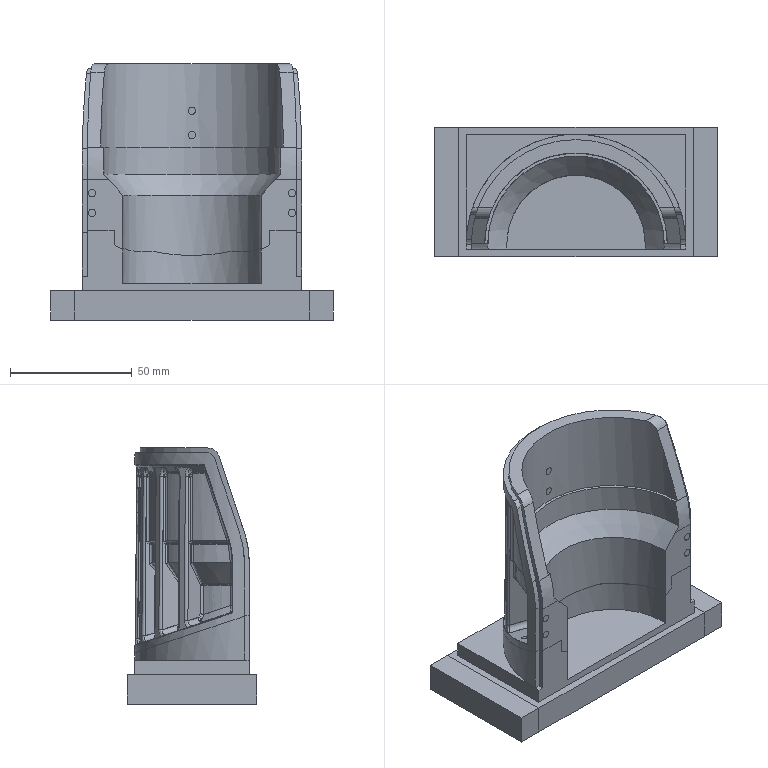NC program | NX | posted by the shop | part box 116 x 53 x 105 mm
Lines 35899 to 37693 of 44585, first 1604 of 1795 lines:
T6 M6
;(T6:C-D4R2  D=4. R=2.)
;(XY=0.05mm Z=0.mm)
G54 G90 D1
G0 A0.0 C=DC(0.0)
CYCLE832(0.04,_TOP_SURFACE_SMOOTH_ON+_ORI_SEMIFIN,1.)
G0 X33.37 Y-1.27 S9000 M3 M8
Z34.1
Z-11.204
G1 Z-12.969 F3500.
X32.577 Y-0. Z-15.797
X33.023 Y-.715 Z-16.056
X33.039 Y-1.129 Z-16.066
X33.046 Y-1.405 Z-16.07
X32.168 Y-0. Z-15.571
X31.759 Z-15.355
X32.401 Y-1.028 Z-15.698
X33.051 Y-2.068 Z-16.073
X33.05 Y-2.328 Z-16.072
X33.044 Y-2.71 Z-16.068
X32.193 Y-1.349 Z-15.585
X31.35 Y-0. Z-15.148
X30.942 Z-14.949
X31.978 Y-1.659 Z-15.47
X33.021 Y-3.328 Z-16.055
X33.012 Y-3.527 Z-16.049
X32.988 Y-3.928 Z-16.035
X32.363 Y-2.929 Z-15.6775
X31.757 Y-1.96 Z-15.355
X30.533 Y-0. Z-14.757
X30.124 Z-14.573
X30.834 Y-1.136 Z-14.898
X31.531 Y-2.252 Z-15.238
X32.2284 Y-3.368 Z-15.604
X32.9433 Y-4.512 Z-16.008
X32.9248 Y-4.726 Z-15.998
X32.8879 Y-5.077 Z-15.976
X32.085 Y-3.792 Z-15.526
X31.299 Y-2.535 Z-15.124
X30.514 Y-1.2774 Z-14.748
X29.715 Y-0. Z-14.396
X29.38 Z-14.277
X29.307 Z-14.259
X29.537 Y-.369 Z-14.3248
X29.755 Y-.718 Z-14.413
X30.191 Y-1.4154 Z-14.603
X31.063 Y-2.811 Z-15.006
X31.935 Y-4.206 Z-15.447
X32.824 Y-5.628 Z-15.9383
X32.785 Y-5.925 Z-15.916
X32.751 Y-6.166 Z-15.896
X31.7784 Y-4.61 Z-15.365
X30.822 Y-3.08 Z-14.893
X29.866 Y-1.55 Z-14.461
X29.627 Y-1.167 Z-14.359
X29.388 Y-.785 Z-14.279
X29.149 Y-.4025 Z-14.231
X28.898 Y-0. Z-14.211
X28.589 Z-14.2284
X28.489 Z-14.244
X28.761 Y-.435 Z-14.213
X29.021 Y-.8507 Z-14.216
X29.28 Y-1.266 Z-14.253
X29.54 Y-1.681 Z-14.326
X30.059 Y-2.512 Z-14.545
X30.578 Y-3.343 Z-14.778
X31.616 Y-5.004 Z-15.281
X32.67 Y-6.691 Z-15.85
X32.582 Y-7.205 Z-15.7998
X31.448 Y-5.39 Z-15.198
X30.3298 Y-3.6 Z-14.666
X29.771 Y-2.7048 Z-14.419
X29.491 Y-2.257 Z-14.309
X29.211 Y-1.81 Z-14.24
X28.932 Y-1.362 Z-14.211
X28.652 Y-.915 Z-14.221
X28.373 Y-.467 Z-14.269
X28.08 Y-0. Z-14.365
X27.997 Z-14.402
X27.799 Z-14.507
X27.672 Y0.0 Z-14.59
X27.722 Y-.08 Z-14.556
X27.834 Y-.259 Z-14.486
X27.983 Y-.499 Z-14.408
X28.283 Y-.978 Z-14.2937
X28.582 Y-1.456 Z-14.229
X28.881 Y-1.935 Z-14.21
X29.18 Y-2.414 Z-14.234
X29.479 Y-2.893 Z-14.303
X30.078 Y-3.851 Z-14.553
X31.275 Y-5.766 Z-15.11
X32.487 Y-7.706 Z-15.746
X32.443 Y-7.923 Z-15.721
X32.385 Y-8.1966 Z-15.689
X31.734 Y-7.154 Z-15.341
X31.098 Y-6.137 Z-15.023
X30.4617 Y-5.119 Z-14.726
X29.826 Y-4.1013 Z-14.444
X29.508 Y-3.592 Z-14.31
X29.19 Y-3.084 Z-14.23
X28.872 Y-2.575 Z-14.207
X28.554 Y-2.066 Z-14.233
X28.236 Y-1.557 Z-14.308
X27.918 Y-1.048 Z-14.44
X27.739 Y-.762 Z-14.545
X27.719 Y-.73 Z-14.558
X27.268 Y-.008 Z-14.859
X27.263 Y0. Z-14.863
X27.262 Y-.652 Z-14.863
X27.72 Y-1.385 Z-14.558
X27.749 Y-1.431 Z-14.539
X27.904 Y-1.681 Z-14.447
X28.216 Y-2.179 Z-14.313
X28.527 Y-2.677 Z-14.232
X28.8382 Y-3.175 Z-14.198
X29.149 Y-3.673 Z-14.216
X29.461 Y-4.171 Z-14.29
X29.772 Y-4.669 Z-14.42
X30.3946 Y-5.666 Z-14.695
X31.017 Y-6.662 Z-14.985
X31.64 Y-7.658 Z-15.293
X32.277 Y-8.679 Z-15.63
X32.164 Y-9.152 Z-15.568
X30.932 Y-7.18 Z-14.944
X29.715 Y-5.233 Z-14.3957
X29.411 Y-4.746 Z-14.269
X29.107 Y-4.259 Z-14.197
X28.803 Y-3.772 Z-14.184
X28.499 Y-3.286 Z-14.222
X28.194 Y-2.799 Z-14.31
X27.89 Y-2.3118 Z-14.452
X27.738 Y-2.068 Z-14.545
X27.695 Y-1.9999 Z-14.574
X27.267 Y-1.314 Z-14.86
X27.262 Y-1.306 Z-14.863
X27.261 Y-1.959 Z-14.864
X27.285 Y-1.998 Z-14.848
X27.5773 Y-2.465 Z-14.646
X27.874 Y-2.94 Z-14.444
X28.171 Y-3.415 Z-14.3
X28.468 Y-3.89 Z-14.206
X28.764 Y-4.365 Z-14.166
X29.061 Y-4.84 Z-14.176
X29.358 Y-5.315 Z-14.246
X29.655 Y-5.79 Z-14.369
X30.842 Y-7.69 Z-14.902
X32.043 Y-9.6127 Z-15.503
X31.96 Y-9.921 Z-15.459
X31.918 Y-10.0668 Z-15.437
X30.746 Y-8.19 Z-14.856
X29.587 Y-6.336 Z-14.3404
X29.298 Y-5.873 Z-14.22
X29.008 Y-5.409 Z-14.1514
X28.719 Y-4.946 Z-14.141
X28.429 Y-4.482 Z-14.186
X28.139 Y-4.019 Z-14.279
X27.85 Y-3.555 Z-14.4313
X27.251 Y-2.597 Z-14.86
X27.249 Y-2.728 Z-14.859
X27.231 Y-3.219 Z-14.8517
X27.532 Y-3.701 Z-14.621
X27.815 Y-4.154 Z-14.409
X28.098 Y-4.606 Z-14.256
X28.381 Y-5.059 Z-14.159
X28.663 Y-5.512 Z-14.114
X28.946 Y-5.964 Z-14.122
X29.2292 Y-6.417 Z-14.191
X29.512 Y-6.87 Z-14.3085
X30.644 Y-8.681 Z-14.808
X31.789 Y-10.514 Z-15.37
X31.728 Y-10.72 Z-15.338
X31.654 Y-10.952 Z-15.3
X30.533 Y-9.1583 Z-14.758
X29.426 Y-7.387 Z-14.272
X29.1497 Y-6.944 Z-14.158
X28.873 Y-6.501 Z-14.09
X28.596 Y-6.058 Z-14.083
X28.32 Y-5.615 Z-14.129
X28.043 Y-5.173 Z-14.23
X27.766 Y-4.73 Z-14.384
X27.195 Y-3.815 Z-14.8377
X27.154 Y-4.326 Z-14.82
X27.147 Y-4.394 Z-14.818
X27.436 Y-4.855 Z-14.578
X27.707 Y-5.2891 Z-14.358
X27.978 Y-5.723 Z-14.197
X28.249 Y-6.156 Z-14.098
X28.52 Y-6.59 Z-14.048
X28.791 Y-7.024 Z-14.055
X29.062 Y-7.4575 Z-14.122
X29.333 Y-7.891 Z-14.233
X30.417 Y-9.626 Z-14.705
X31.515 Y-11.3827 Z-15.229
X31.47 Y-11.52 Z-15.207
X31.371 Y-11.8072 Z-15.158
X30.295 Y-10.085 Z-14.65
X29.232 Y-8.384 Z-14.191
X28.966 Y-7.959 Z-14.083
X28.701 Y-7.534 Z-14.017
X28.435 Y-7.109 Z-14.013
X28.169 Y-6.684 Z-14.061
X27.9038 Y-6.258 Z-14.165
X27.638 Y-5.833 Z-14.3247
X27.372 Y-5.408 Z-14.5505
X27.09 Y-4.956 Z-14.796
X27.07 Y-5.126 Z-14.788
X27.0224 Y-5.502 Z-14.77
X27.3 Y-5.946 Z-14.518
X27.56 Y-6.363 Z-14.29
X27.821 Y-6.78 Z-14.127
X28.082 Y-7.1971 Z-14.0235
X28.342 Y-7.614 Z-13.972
X28.603 Y-8.031 Z-13.977
X28.864 Y-8.448 Z-14.042
X29.124 Y-8.865 Z-14.147
X30.167 Y-10.534 Z-14.592
X31.223 Y-12.224 Z-15.084
X31.07 Y-12.634 Z-15.01
X30.033 Y-10.974 Z-14.534
X29.009 Y-9.335 Z-14.1007
X28.7525 Y-8.9248 Z-13.999
X28.496 Y-8.515 Z-13.935
X28.2404 Y-8.105 Z-13.932
X27.984 Y-7.696 Z-13.982
X27.728 Y-7.286 Z-14.089
X27.472 Y-6.876 Z-14.255
X27.216 Y-6.466 Z-14.484
X26.944 Y-6.031 Z-14.74
X26.898 Y-6.325 Z-14.7225
X26.857 Y-6.5456 Z-14.707
X27.125 Y-6.974 Z-14.451
X27.376 Y-7.3766 Z-14.215
X27.628 Y-7.78 Z-14.049
X27.88 Y-8.182 Z-13.941
X28.132 Y-8.585 Z-13.887
X28.383 Y-8.988 Z-13.8903
X28.635 Y-9.391 Z-13.953
X28.887 Y-9.794 Z-14.053
X29.894 Y-11.406 Z-14.4743
X30.914 Y-13.039 Z-14.936
X30.754 Y-13.436 Z-14.86
X29.751 Y-11.83 Z-14.412
X28.76 Y-10.246 Z-14.003
X28.513 Y-9.85 Z-13.906
X28.2654 Y-9.4535 Z-13.844
X28.018 Y-9.057 Z-13.843
X27.77 Y-8.661 Z-13.896
X27.523 Y-8.265 Z-14.004
X27.275 Y-7.869 Z-14.176
X27.028 Y-7.4728 Z-14.41
X26.764 Y-7.051 Z-14.672
X26.7512 Y-7.124 Z-14.668
X26.664 Y-7.545 Z-14.635
X26.923 Y-7.959 Z-14.369
X27.167 Y-8.349 Z-14.129
X27.41 Y-8.739 Z-13.96
X27.654 Y-9.129 Z-13.849
X27.897 Y-9.519 Z-13.7945
X28.141 Y-9.909 Z-13.796
X28.385 Y-10.298 Z-13.857
X28.628 Y-10.688 Z-13.952
X29.603 Y-12.248 Z-14.348
X30.59 Y-13.828 Z-14.784
X30.422 Y-14.214 Z-14.707
X29.45 Y-12.657 Z-14.284
X28.49 Y-11.12 Z-13.897
X28.25 Y-10.736 Z-13.806
X28.01 Y-10.352 Z-13.746
X27.77 Y-9.9682 Z-13.747
X27.53 Y-9.5841 Z-13.802
X27.29 Y-9.2 Z-13.912
X27.05 Y-8.816 Z-14.0872
X26.81 Y-8.432 Z-14.327
X26.555 Y-8.024 Z-14.596
X26.438 Y-8.492 Z-14.553
X26.69 Y-8.894 Z-14.285
X26.9262 Y-9.273 Z-14.039
X27.163 Y-9.651 Z-13.867
X27.399 Y-10.03 Z-13.753
X27.636 Y-10.409 Z-13.696
X27.873 Y-10.787 Z-13.695
X28.109 Y-11.1662 Z-13.754
X28.346 Y-11.545 Z-13.843
X29.293 Y-13.06 Z-14.218
X30.252 Y-14.595 Z-14.631
X30.17 Y-14.776 Z-14.594
X30.078 Y-14.9706 Z-14.554
X29.132 Y-13.457 Z-14.154
X28.198 Y-11.9627 Z-13.788
X27.965 Y-11.589 Z-13.701
X27.732 Y-11.216 Z-13.643
X27.498 Y-10.842 Z-13.645
X27.2649 Y-10.469 Z-13.702
X27.032 Y-10.095 Z-13.815
X26.798 Y-9.722 Z-13.993
X26.565 Y-9.348 Z-14.237
X26.317 Y-8.952 Z-14.512
X26.271 Y-9.122 Z-14.493
X26.19 Y-9.402 Z-14.464
X26.434 Y-9.793 Z-14.1896
X26.664 Y-10.162 Z-13.941
X26.895 Y-10.53 Z-13.766
X27.125 Y-10.899 Z-13.65
X27.355 Y-11.267 Z-13.591
X27.585 Y-11.635 Z-13.589
X27.815 Y-12.004 Z-13.646
X28.046 Y-12.372 Z-13.731
X28.966 Y-13.846 Z-14.089
X29.9 Y-15.339 Z-14.476
X29.7191 Y-15.705 Z-14.399
X28.7979 Y-14.23 Z-14.02
X27.889 Y-12.776 Z-13.674
X27.662 Y-12.412 Z-13.591
X27.435 Y-12.049 Z-13.535
X27.207 Y-11.685 Z-13.538
X26.98 Y-11.322 Z-13.597
X26.753 Y-10.9579 Z-13.712
X26.526 Y-10.5943 Z-13.891
X26.299 Y-10.2307 Z-14.14
X26.057 Y-9.845 Z-14.419
X25.92 Y-10.278 Z-14.371
X26.158 Y-10.66 Z-14.089
X26.382 Y-11.019 Z-13.837
X26.607 Y-11.378 Z-13.659
X26.831 Y-11.737 Z-13.542
X27.055 Y-12.096 Z-13.4826
X27.28 Y-12.455 Z-13.479
X27.504 Y-12.814 Z-13.535
X27.728 Y-13.173 Z-13.617
X28.626 Y-14.609 Z-13.951
X29.535 Y-16.064 Z-14.321
X29.349 Y-16.42 Z-14.243
X28.45 Y-14.981 Z-13.883
X27.5628 Y-13.562 Z-13.556
X27.341 Y-13.207 Z-13.477
X27.119 Y-12.852 Z-13.423
X26.898 Y-12.497 Z-13.428
X26.676 Y-12.143 Z-13.487
X26.454 Y-11.788 Z-13.604
X26.232 Y-11.433 Z-13.786
X26.011 Y-11.078 Z-14.039
X25.775 Y-10.702 Z-14.32
X25.625 Y-11.116 Z-14.27
X25.8581 Y-11.488 Z-13.988
X26.0773 Y-11.839 Z-13.731
X26.296 Y-12.19 Z-13.55
X26.516 Y-12.54 Z-13.432
X26.735 Y-12.891 Z-13.37
X26.954 Y-13.242 Z-13.365
X27.173 Y-13.593 Z-13.419
X27.392 Y-13.944 Z-13.495
X28.269 Y-15.347 Z-13.817
X29.158 Y-16.769 Z-14.165
X28.965 Y-17.115 Z-14.087
X28.087 Y-15.7087 Z-13.75
X27.22 Y-14.322 Z-13.435
X27.003 Y-13.975 Z-13.36
X26.787 Y-13.628 Z-13.3076
X26.733 Y-13.542 Z-13.304
X26.678 Y-13.455 Z-13.303
X26.57 Y-13.282 Z-13.3131
X26.353 Y-12.935 Z-13.3738
X26.137 Y-12.588 Z-13.4922
X25.92 Y-12.241 Z-13.677
X25.704 Y-11.895 Z-13.9316
X25.474 Y-11.527 Z-14.2193
X25.314 Y-11.926 Z-14.166
X25.542 Y-12.29 Z-13.879
X25.756 Y-12.633 Z-13.619
X25.9703 Y-12.976 Z-13.436
X26.077 Y-13.147 Z-13.37
X26.131 Y-13.233 Z-13.342
X26.185 Y-13.319 Z-13.318
X26.399 Y-13.662 Z-13.255
X26.613 Y-14.005 Z-13.249
X26.828 Y-14.3481 Z-13.3003
X27.042 Y-14.691 Z-13.374
X27.9 Y-16.064 Z-13.679
X28.769 Y-17.455 Z-14.008
X28.571 Y-17.793 Z-13.93
X27.711 Y-16.415 Z-13.609
X26.65 Y-14.7176 Z-13.24
X26.438 Y-14.378 Z-13.19
X26.226 Y-14.038 Z-13.197
X26.013 Y-13.699 Z-13.26
X25.801 Y-13.359 Z-13.379
X25.695 Y-13.19 Z-13.463
X25.642 Y-13.1047 Z-13.512
X25.589 Y-13.02 Z-13.565
X25.377 Y-12.68 Z-13.822
X25.152 Y-12.3201 Z-14.113
X24.984 Y-12.706 Z-14.059
X25.207 Y-13.063 Z-13.768
X25.417 Y-13.399 Z-13.508
X25.627 Y-13.735 Z-13.322
X25.837 Y-14.071 Z-13.2015
X25.942 Y-14.239 Z-13.163
X25.995 Y-14.3233 Z-13.149
X26.047 Y-14.407 Z-13.139
X26.257 Y-14.743 Z-13.132
X26.467 Y-15.079 Z-13.1815
X26.677 Y-15.416 Z-13.25
X27.517 Y-16.76 Z-13.54
X28.369 Y-18.123 Z-13.853
X28.253 Y-18.313 Z-13.808
X28.165 Y-18.451 Z-13.776
X27.321 Y-17.1001 Z-13.4718
X26.489 Y-15.7679 Z-13.188
X26.281 Y-15.435 Z-13.125
X26.0726 Y-15.1018 Z-13.077
X25.864 Y-14.769 Z-13.083
X25.656 Y-14.436 Z-13.145
X25.448 Y-14.103 Z-13.2659
X25.396 Y-14.019 Z-13.306
X25.3442 Y-13.936 Z-13.35
X25.24 Y-13.77 Z-13.452
X25.032 Y-13.437 Z-13.715
X24.811 Y-13.083 Z-14.007
X24.633 Y-13.453 Z-13.958
X24.852 Y-13.803 Z-13.664
X25.058 Y-14.133 Z-13.399
X25.265 Y-14.4632 Z-13.211
X25.471 Y-14.793 Z-13.091
X25.678 Y-15.124 Z-13.028
X25.884 Y-15.454 Z-13.021
X26.0902 Y-15.784 Z-13.068
X26.297 Y-16.1143 Z-13.13
X27.122 Y-17.435 Z-13.403
X27.959 Y-18.775 Z-13.699
X27.75 Y-19.0945 Z-13.622
X26.919 Y-17.764 Z-13.332
X26.0991 Y-16.452 Z-13.073
X25.689 Y-15.797 Z-12.97
X25.484 Y-15.469 Z-12.977
X25.279 Y-15.141 Z-13.0398
X25.075 Y-14.813 Z-13.1618
X24.87 Y-14.485 Z-13.35
X24.665 Y-14.157 Z-13.619
X24.448 Y-13.809 Z-13.917
X24.391 Y-13.917 Z-13.905
X24.259 Y-14.162 Z-13.878
X24.475 Y-14.508 Z-13.574
X24.678 Y-14.833 Z-13.305
X24.882 Y-15.1585 Z-13.114
X25.085 Y-15.484 Z-12.992
X25.289 Y-15.809 Z-12.929
X25.492 Y-16.135 Z-12.922
X25.899 Y-16.786 Z-13.017
X26.712 Y-18.088 Z-13.261
X27.538 Y-19.408 Z-13.546
X27.404 Y-19.606 Z-13.499
X27.323 Y-19.7197 Z-13.47
X26.503 Y-18.407 Z-13.194
X25.694 Y-17.113 Z-12.964
X25.2899 Y-16.466 Z-12.876
X25.088 Y-16.142 Z-12.884
X24.886 Y-15.819 Z-12.948
X24.683 Y-15.495 Z-13.0716
X24.481 Y-15.1714 Z-13.264
X24.279 Y-14.848 Z-13.539
X24.065 Y-14.505 Z-13.845
X23.943 Y-14.717 Z-13.824
X23.867 Y-14.843 Z-13.813
X24.08 Y-15.184 Z-13.504
X24.281 Y-15.506 Z-13.2263
X24.4823 Y-15.827 Z-13.031
X24.683 Y-16.149 Z-12.907
X24.884 Y-16.471 Z-12.842
X25.085 Y-16.7922 Z-12.834
X25.487 Y-17.435 Z-12.916
X26.291 Y-18.722 Z-13.132
X27.106 Y-20.027 Z-13.395
X27.009 Y-20.165 Z-13.362
X26.887 Y-20.331 Z-13.32
X26.077 Y-19.0335 Z-13.066
X25.278 Y-17.755 Z-12.872
X24.878 Y-17.115 Z-12.795
X24.679 Y-16.796 Z-12.8035
X24.479 Y-16.4758 Z-12.869
X24.279 Y-16.156 Z-12.994
X24.079 Y-15.836 Z-13.19
X23.879 Y-15.517 Z-13.471
X23.6678 Y-15.178 Z-13.784
X23.466 Y-15.509 Z-13.757
X23.676 Y-15.845 Z-13.44
X23.875 Y-16.163 Z-13.157
X24.073 Y-16.481 Z-12.96
X24.272 Y-16.798 Z-12.834
X24.47 Y-17.116 Z-12.768
X24.668 Y-17.434 Z-12.759
X25.065 Y-18.0688 Z-12.832
X25.8594 Y-19.339 Z-13.006
X26.6647 Y-20.628 Z-13.245
X26.613 Y-20.697 Z-13.228
X26.429 Y-20.905 Z-13.17
X25.631 Y-19.628 Z-12.95
X24.844 Y-18.369 Z-12.788
X24.451 Y-17.739 Z-12.728
X24.254 Y-17.425 Z-12.738
X24.057 Y-17.11 Z-12.804
X23.861 Y-16.795 Z-12.932
X23.664 Y-16.48 Z-13.131
X23.467 Y-16.165 Z-13.417
X23.259 Y-15.832 Z-13.737
X23.05 Y-16.151 Z-13.7183
X23.256 Y-16.482 Z-13.3973
X23.451 Y-16.793 Z-13.108
X23.646 Y-17.105 Z-12.907
X23.841 Y-17.417 Z-12.778
X24.035 Y-17.729 Z-12.711
X24.23 Y-18.041 Z-12.7
X24.62 Y-18.664 Z-12.752
X25.399 Y-19.911 Z-12.903
X25.789 Y-20.535 Z-12.9873
X26.19 Y-21.176 Z-13.097
X25.947 Y-21.441 Z-13.03
X25.164 Y-20.188 Z-12.85
X24.392 Y-18.953 Z-12.721
X24.006 Y-18.3354 Z-12.676
X23.813 Y-18.027 Z-12.688
X23.62 Y-17.718 Z-12.757
X23.427 Y-17.409 Z-12.887
X23.234 Y-17.1 Z-13.09
X23.041 Y-16.791 Z-13.3806
X22.836 Y-16.464 Z-13.706
X22.662 Y-16.72 Z-13.696
X22.622 Y-16.775 Z-13.695
X22.824 Y-17.099 Z-13.368
X23.016 Y-17.405 Z-13.074
X23.2067 Y-17.7106 Z-12.87
X23.398 Y-18.016 Z-12.74
X23.589 Y-18.322 Z-12.6693
X23.78 Y-18.628 Z-12.655
X24.162 Y-19.24 Z-12.695
X24.927 Y-20.463 Z-12.802
X25.702 Y-21.704 Z-12.966
X25.456 Y-21.964 Z-12.9082
X24.687 Y-20.733 Z-12.762
X23.929 Y-19.521 Z-12.6678
X23.55 Y-18.914 Z-12.639
X23.361 Y-18.611 Z-12.655
X23.171 Y-18.308 Z-12.727
X22.982 Y-18.005 Z-12.859
X22.792 Y-17.701 Z-13.066
X22.603 Y-17.398 Z-13.361
X22.402 Y-17.077 Z-13.692
X22.181 Y-17.377 Z-13.691
X22.38 Y-17.696 Z-13.358
X22.568 Y-17.996 Z-13.059
X22.756 Y-18.297 Z-12.851
X22.943 Y-18.597 Z-12.718
X23.131 Y-18.898 Z-12.645
X23.319 Y-19.198 Z-12.627
X23.694 Y-19.799 Z-12.649
X24.445 Y-21. Z-12.731
X25.207 Y-22.2192 Z-12.855
X25.033 Y-22.396 Z-12.821
X24.956 Y-22.472 Z-12.807
X24.201 Y-21.264 Z-12.699
X23.457 Y-20.073 Z-12.634
X23.085 Y-19.478 Z-12.62
X22.899 Y-19.18 Z-12.639
X22.713 Y-18.883 Z-12.713
X22.527 Y-18.585 Z-12.847
X22.341 Y-18.287 Z-13.057
X22.155 Y-17.99 Z-13.359
X21.957 Y-17.674 Z-13.694
X21.772 Y-17.914 Z-13.7005
X21.731 Y-17.965 Z-13.703
X22.065 Y-18.4998 Z-13.127
X22.203 Y-18.721 Z-12.943
X22.342 Y-18.942 Z-12.8082
X22.48 Y-19.164 Z-12.713
X22.664 Y-19.4589 Z-12.638
X22.849 Y-19.754 Z-12.617
X23.217 Y-20.344 Z-12.625
X23.955 Y-21.525 Z-12.671
X24.704 Y-22.722 Z-12.765
X24.448 Y-22.968 Z-12.728
X23.706 Y-21.781 Z-12.649
X22.975 Y-20.611 Z-12.618
X22.8213 Y-20.364 Z-12.617
X22.601 Y-20.013
X22.564 Y-19.953 Z-12.618
X22.519 Y-19.88 Z-12.622
X22.427 Y-19.734 Z-12.64
X22.245 Y-19.4415 Z-12.716
X22.062 Y-19.1491 Z-12.8536
X22.016 Y-19.076 Z-12.899
X21.971 Y-19.003 Z-12.949
X21.879 Y-18.857 Z-13.066
X21.6965 Y-18.564 Z-13.371
X21.503 Y-18.254 Z-13.713
X21.274 Y-18.543 Z-13.718
X21.467 Y-18.85 Z-13.3763
X21.647 Y-19.14 Z-13.071
X21.828 Y-19.43 Z-12.858
X22.009 Y-19.719 Z-12.72
X22.19 Y-20.009 Z-12.642
X22.281 Y-20.153 Z-12.623
X22.3599 Y-20.28 Z-12.617
X22.371 Y-20.298 Z-12.617
X22.824 Y-21.022
X23.095 Y-21.456 Z-12.62
X23.4568 Y-22.035 Z-12.636
X24.191 Y-23.211 Z-12.695
X23.932 Y-23.451 Z-12.67
X23.205 Y-22.287 Z-12.623
X22.822 Y-21.674 Z-12.617
X22.134 Y-20.573
X21.952 Y-20.281 Z-12.643
X21.773 Y-19.995 Z-12.721
X21.594 Y-19.708 Z-12.86
X21.415 Y-19.422 Z-13.075
X21.236 Y-19.135 Z-13.38
X21.046 Y-18.831 Z-13.718
X20.813 Y-19.113 Z-13.717
X21.002 Y-19.415 Z-13.378
X21.179 Y-19.698 Z-13.075
X21.356 Y-19.982 Z-12.862
X21.533 Y-20.266 Z-12.724
X21.711 Y-20.549 Z-12.644
X21.896 Y-20.846 Z-12.617
X21.899 Y-20.8509
X22.8216 Y-22.327
X22.952 Y-22.536 Z-12.618
X23.672 Y-23.688 Z-12.647
X23.41 Y-23.9228 Z-12.6317
X23.048 Y-23.343 Z-12.62
X22.823 Y-22.983 Z-12.617
X21.662 Y-21.125
X21.642 Y-21.094 Z-12.617
X21.467 Y-20.8129 Z-12.647
X21.291 Y-20.532 Z-12.7275
X21.115 Y-20.251 Z-12.867
X20.94 Y-19.969 Z-13.079
X20.7639 Y-19.688 Z-13.381
X20.5771 Y-19.389 Z-13.717
X20.341 Y-19.666 Z-13.717
X20.526 Y-19.962 Z-13.384
X20.7 Y-20.24 Z-13.085
X20.874 Y-20.518 Z-12.872
X21.048 Y-20.797 Z-12.732
X21.222 Y-21.075 Z-12.6494
X21.396 Y-21.353 Z-12.617
X21.423 Y-21.3967 Z-12.617
X22.822 Y-23.636
X23.145 Y-24.153 Z-12.621
X22.968 Y-24.308 Z-12.6185
X22.8824 Y-24.387 Z-12.617
X22.823 Y-24.292 Z-12.617
X21.176 Y-21.656
X21.149 Y-21.613 Z-12.617
X20.9767 Y-21.337 Z-12.649
X20.804 Y-21.061 Z-12.732
X20.632 Y-20.786 Z-12.873
X20.46 Y-20.51 Z-13.088
X20.288 Y-20.234 Z-13.3886
X20.104 Y-19.941 Z-13.719
X19.862 Y-20.207 Z-13.717
X20.044 Y-20.499 Z-13.384
X20.216 Y-20.773 Z-13.085
X20.387 Y-21.047 Z-12.872
X20.5581 Y-21.321 Z-12.732
X20.729 Y-21.595 Z-12.649
X20.901 Y-21.869 Z-12.617
X20.93 Y-21.917 Z-12.617
X22.621 Y-24.623
X22.624 Y-24.628
X22.371 Y-24.876
X20.684 Y-22.176
X20.652 Y-22.1249 Z-12.617
X20.481 Y-21.852 Z-12.65
X20.31 Y-21.578 Z-12.733
X20.139 Y-21.305 Z-12.873
X19.968 Y-21.031 Z-13.086
X19.797 Y-20.758 Z-13.385
X19.6156 Y-20.467 Z-13.717
X19.369 Y-20.727 Z-13.7173
X19.55 Y-21.017 Z-13.386
X19.721 Y-21.29 Z-13.087
X19.891 Y-21.562 Z-12.875
X20.062 Y-21.835 Z-12.734
X20.232 Y-22.107 Z-12.651
X20.402 Y-22.38 Z-12.618
X20.437 Y-22.4355 Z-12.617
X22.117 Y-25.124
X21.857 Y-25.362
X20.182 Y-22.682
X20.151 Y-22.632 Z-12.617
X19.981 Y-22.36 Z-12.65
X19.812 Y-22.089 Z-12.733
X19.642 Y-21.818 Z-12.8738
X19.473 Y-21.546 Z-13.088
X19.303 Y-21.2752 Z-13.388
X19.123 Y-20.9864 Z-13.717
X18.999 Y-21.111 Z-13.717
X18.869 Y-21.234 Z-13.717
X19.049 Y-21.522 Z-13.384
X19.2179 Y-21.793 Z-13.085
X19.387 Y-22.064 Z-12.8723
X19.556 Y-22.334 Z-12.732
X19.725 Y-22.605 Z-12.65
X19.894 Y-22.876 Z-12.617
X19.9261 Y-22.926 Z-12.617
X21.596 Y-25.599
X21.336 Y-25.837
X19.668 Y-23.168
X19.636 Y-23.117 Z-12.617
X19.468 Y-22.847 Z-12.65
X19.299 Y-22.576 Z-12.733
X19.13 Y-22.306 Z-12.873
X18.961 Y-22.036 Z-13.086
X18.792 Y-21.765 Z-13.385
X18.612 Y-21.478 Z-13.717
X18.356 Y-21.721 Z-13.717
X18.535 Y-22.008 Z-13.3853
X18.7038 Y-22.278 Z-13.086
X18.872 Y-22.548 Z-12.874
X19.041 Y-22.818 Z-12.733
X19.21 Y-23.0882 Z-12.65
X19.378 Y-23.358 Z-12.617
X19.41 Y-23.409 Z-12.617
X21.0759 Y-26.075
X20.81 Y-26.303
X19.149 Y-23.645
X19.118 Y-23.595 Z-12.617
X18.95 Y-23.326 Z-12.65
X18.781 Y-23.057 Z-12.733
X18.6132 Y-22.788 Z-12.874
X18.445 Y-22.518 Z-13.089
X18.277 Y-22.249 Z-13.388
X18.098 Y-21.963 Z-13.719
X17.919 Y-22.124 Z-13.718
X17.835 Y-22.196 Z-13.718
X18.014 Y-22.482 Z-13.384
X18.181 Y-22.75 Z-13.084
X18.349 Y-23.019 Z-12.872
X18.517 Y-23.288 Z-12.732
X18.685 Y-23.556 Z-12.649
X18.853 Y-23.825 Z-12.617
X18.884 Y-23.875 Z-12.617
X20.541 Y-26.527
X20.374 Y-26.667
X20.22
X18.616 Y-24.101
X18.565 Y-24.018 Z-12.619
X18.4006 Y-23.756 Z-12.655
X18.236 Y-23.493 Z-12.741
X18.072 Y-23.23 Z-12.883
X17.908 Y-22.967 Z-13.095
X17.569 Y-22.4239 Z-13.7175
X17.302 Y-22.652 Z-13.717
X17.624 Y-23.166 Z-13.124
X17.779 Y-23.415 Z-12.912
X17.934 Y-23.663 Z-12.767
X18.09 Y-23.912 Z-12.674
X18.245 Y-24.1607 Z-12.625
X18.323 Y-24.285 Z-12.617
X18.347 Y-24.324 Z-12.617
X19.811 Y-26.667
X19.402
X18.08 Y-24.55
X17.924 Y-24.301 Z-12.637
X17.777 Y-24.066 Z-12.695
X17.631 Y-23.832 Z-12.795
X17.484 Y-23.597 Z-12.945
X17.338 Y-23.363 Z-13.156
X17.034 Y-22.876 Z-13.721
X16.762 Y-23.095 Z-13.7177
X17.049 Y-23.554 Z-13.18
X17.187 Y-23.775 Z-12.971
X17.325 Y-23.996 Z-12.821
X17.463 Y-24.217 Z-12.717
X17.6009 Y-24.438 Z-12.651
X17.739 Y-24.659 Z-12.62
X17.804 Y-24.763 Z-12.617
X18.994 Y-26.667
X18.585
X17.527 Y-24.973
X17.47 Y-24.882 Z-12.619
X17.4049 Y-24.7785 Z-12.629
X17.275 Y-24.571 Z-12.671
X17.1454 Y-24.3632 Z-12.744
X17.016 Y-24.156 Z-12.852
X16.886 Y-23.9479 Z-13.003
X16.756 Y-23.74 Z-13.209
X16.486 Y-23.308 Z-13.717
X16.21 Y-23.52 Z-13.717
X16.463 Y-23.926 Z-13.241
X16.585 Y-24.12 Z-13.038
X16.706 Y-24.314 Z-12.887
X16.828 Y-24.509 Z-12.774
X16.949 Y-24.7032 Z-12.695
X17.0706 Y-24.898 Z-12.644
X17.192 Y-25.092 Z-12.619
X17.249 Y-25.183 Z-12.617
X18.176 Y-26.667
X17.768 Y-26.667
X16.973 Y-25.396
X16.849 Y-25.198 Z-12.629
X16.736 Y-25.017 Z-12.665
X16.623 Y-24.835 Z-12.724
X16.51 Y-24.654 Z-12.809
X16.397 Y-24.473 Z-12.924
X16.283 Y-24.2918 Z-13.075
X16.17 Y-24.111 Z-13.272
X15.933 Y-23.731 Z-13.718
X15.652 Y-23.936 Z-13.717
X15.873 Y-24.29 Z-13.299
X15.978 Y-24.458 Z-13.108
X16.084 Y-24.626 Z-12.958
X16.189 Y-24.795 Z-12.842
X16.294 Y-24.9632 Z-12.754
X16.399 Y-25.132 Z-12.689
X16.505 Y-25.3 Z-12.645
X16.61 Y-25.468 Z-12.622
X16.685 Y-25.589 Z-12.617
X17.359 Y-26.667
X16.95
X16.402 Y-25.79
X16.3531 Y-25.7117 Z-12.618
X16.158 Y-25.4 Z-12.667
X15.963 Y-25.088 Z-12.788
X15.8659 Y-24.932 Z-12.88
X15.768 Y-24.776 Z-12.996
X15.671 Y-24.62 Z-13.144
X15.574 Y-24.464 Z-13.325
X15.368 Y-24.135 Z-13.717
X15.253 Y-24.216 Z-13.717
X15.3 Y-24.4581 Z-13.489
X15.231 Y-24.569 Z-13.435
X15.403 Y-24.846 Z-13.113
X15.564 Y-25.103 Z-12.897
X15.725 Y-25.36 Z-12.752
X15.886 Y-25.618 Z-12.662
X16.047 Y-25.875 Z-12.62
X16.117 Y-25.988 Z-12.617
X16.541 Y-26.667
X16.132
X15.8287 Y-26.1807
X15.782 Y-26.1063 Z-12.6184
X15.7146 Y-25.9981 Z-12.628
X15.579 Y-25.782 Z-12.6705
X15.444 Y-25.565 Z-12.748
X15.309 Y-25.349 Z-12.864
X15.174 Y-25.132 Z-13.028
X15.033 Y-24.907 Z-13.266
X15.027 Y-24.897 Z-13.2722
X14.894 Y-25.107 Z-13.175
X14.817 Y-25.215 Z-13.128
X14.828 Y-25.233 Z-13.1093
X14.938 Y-25.41 Z-12.953
X15.049 Y-25.587 Z-12.833
X15.159 Y-25.764 Z-12.743
X15.27 Y-25.94 Z-12.678
X15.38 Y-26.117 Z-12.637
X15.491 Y-26.294 Z-12.618
X15.536 Y-26.366 Z-12.617
X15.724 Y-26.667
X15.315 Y-26.667
X15.241 Y-26.549
X15.217 Y-26.51 Z-12.617
X15.132 Y-26.373 Z-12.627
X14.96 Y-26.0991 Z-12.685
X14.789 Y-25.825 Z-12.801
X14.618 Y-25.551 Z-12.985
X14.606 Y-25.5316 Z-13.001
X14.4106 Y-25.874 Z-12.88
X14.423 Y-25.893 Z-12.868
X14.5405 Y-26.081 Z-12.763
X14.658 Y-26.27 Z-12.689
X14.776 Y-26.459 Z-12.641
X14.904 Y-26.663 Z-12.618
X14.907 Y-26.667 Z-12.617
X14.079 Y-25.343 Z-9.824
Z-8.5
G0 Z34.1
X-26.932 Y-1.1693
Z-11.104
G1 Z-11.708
X-27.663 Y-0. Z-14.595
X-27.267 Y-.634 Z-14.8599
X-27.262 Y-.642 Z-14.863
X-27.262 Y-1.2842 Z-14.863
X-27.721 Y-.549 Z-14.557
X-27.763 Y-.482 Z-14.529
X-27.859 Y-.328 Z-14.472
X-28.0642 Y-0. Z-14.372
X-28.192 Z-14.3226
X-28.39 Z-14.265
X-28.465 Z-14.249
X-28.16 Y-.489 Z-14.334
X-27.867 Y-.957 Z-14.468
X-27.757 Y-1.133 Z-14.533
X-27.721 Y-1.191 Z-14.557
X-27.267 Y-1.918 Z-14.86
X-27.262 Y-1.926 Z-14.863
X-27.258 Y-2.328 Z-14.862
X-27.252 Y-2.584 Z-14.862
X-27.619 Y-1.997 Z-14.625
X-27.719 Y-1.836 Z-14.558
X-27.816 Y-1.681 Z-14.497
X-27.965 Y-1.4434 Z-14.417
X-28.261 Y-.969 Z-14.3
X-28.557 Y-.494 Z-14.233
X-28.866 Y-0. Z-14.21
X-28.983 Z-14.214
X-29.268 Z-14.251
X-29.004 Y-.421 Z-14.215
X-28.753 Y-.823 Z-14.213
X-28.503 Y-1.224 Z-14.242
X-28.252 Y-1.626 Z-14.303
X-28.001 Y-2.027 Z-14.399
X-27.75 Y-2.428 Z-14.5299
X-27.227 Y-3.2661 Z-14.851
X-27.214 Y-3.527 Z-14.845
X-27.18 Y-3.982 Z-14.832
X-27.8163 Y-2.964 Z-14.477
X-28.123 Y-2.474 Z-14.341
X-28.4296 Y-1.983 Z-14.256
X-28.736 Y-1.492 Z-14.2141
X-29.043 Y-1.002 Z-14.218
X-29.35 Y-.511 Z-14.269
X-29.6687 Y-0. Z-14.376
X-30.07 Z-14.549
X-29.693 Y-.604 Z-14.386
X-29.328 Y-1.187 Z-14.264
X-28.963 Y-1.7707 Z-14.2128
X-28.599 Y-2.354 Z-14.224
X-28.234 Y-2.938 Z-14.295
X-27.869 Y-3.521 Z-14.421
X-27.116 Y-4.727 Z-14.806
X-27.071 Y-5.126 Z-14.789
X-27.02 Y-5.522 Z-14.768
X-27.472 Y-4.799 Z-14.56
X-27.899 Y-4.116 Z-14.369
X-28.3254 Y-3.434 Z-14.253
X-28.752 Y-2.751 Z-14.207
X-28.965 Y-2.41 Z-14.21
X-29.179 Y-2.068 Z-14.235
X-29.392 Y-1.727 Z-14.28
X-29.605 Y-1.385 Z-14.35
X-30.471 Y-0. Z-14.729
X-30.872 Z-14.915
X-29.874 Y-1.598 Z-14.464
X-29.627 Y-1.993 Z-14.359
X-29.381 Y-2.387 Z-14.276
X-29.134 Y-2.782 Z-14.224
X-28.887 Y-3.176 Z-14.198
X-28.641 Y-3.571 Z-14.197
X-28.394 Y-3.965 Z-14.216
X-28.148 Y-4.36 Z-14.256
X-27.901 Y-4.754 Z-14.318
X-27.655 Y-5.149 Z-14.4
X-27.408 Y-5.543 Z-14.507
X-26.887 Y-6.377 Z-14.718
X-26.826 Y-6.724 Z-14.695
X-26.75 Y-7.124 Z-14.666
X-26.715 Y-7.2946 Z-14.6537
X-27.31 Y-6.343 Z-14.446
X-27.592 Y-5.891 Z-14.34
X-27.874 Y-5.44 Z-14.265
X-28.156 Y-4.988 Z-14.21
X-28.439 Y-4.536 Z-14.181
X-28.721 Y-4.085 Z-14.175
X-29.003 Y-3.6331 Z-14.197
X-29.285 Y-3.181 Z-14.248
X-29.567 Y-2.73 Z-14.335
X-30.132 Y-1.827 Z-14.577
X-31.273 Y-0. Z-15.11
X-31.674 Z-15.311
X-31.019 Y-1.049 Z-14.985
X-30.376 Y-2.078 Z-14.687
X-29.733 Y-3.1065 Z-14.403
X-29.412 Y-3.621 Z-14.278
X-29.0903 Y-4.135 Z-14.197
X-28.769 Y-4.65 Z-14.155
X-28.447 Y-5.164 Z-14.143
X-28.126 Y-5.679 Z-14.161
X-27.805 Y-6.193 Z-14.2056
X-27.4831 Y-6.7074 Z-14.275
X-27.162 Y-7.222 Z-14.376
X-26.485 Y-8.304 Z-14.569
X-26.381 Y-8.722 Z-14.533
X-26.272 Y-9.122 Z-14.493
X-26.183 Y-9.43 Z-14.463
X-26.952 Y-8.2 Z-14.291
X-27.317 Y-7.615 Z-14.201
X-27.682 Y-7.031 Z-14.14
X-28.047 Y-6.447 Z-14.1069
X-28.412 Y-5.8626 Z-14.101
X-28.7772 Y-5.278 Z-14.128
X-29.142 Y-4.694 Z-14.195
X-29.507 Y-4.11 Z-14.308
X-29.872 Y-3.526 Z-14.463
X-30.603 Y-2.357 Z-14.789
X-31.333 Y-1.189 Z-15.1399
X-32.075 Y-0. Z-15.521
X-32.477 Z-15.74
X-31.631 Y-1.353 Z-15.288
X-30.7976 Y-2.687 Z-14.881
X-29.964 Y-4.02 Z-14.5031
X-29.548 Y-4.687 Z-14.323
X-29.131 Y-5.354 Z-14.178
X-28.7145 Y-6.021 Z-14.09
X-28.298 Y-6.687 Z-14.047
X-27.881 Y-7.354 Z-14.041
X-27.465 Y-8.021 Z-14.064
X-27.048 Y-8.688 Z-14.115
X-26.631 Y-9.354 Z-14.191
X-26.215 Y-10.021 Z-14.261
X-25.7499 Y-10.765 Z-14.313
X-25.625 Y-11.12 Z-14.271
X-25.477 Y-11.52 Z-14.22
X-25.318 Y-11.919 Z-14.1677
X-25.084 Y-12.472 Z-14.091
X-25.154 Y-12.361 Z-14.0927
X-25.636 Y-11.589 Z-14.092
X-26.118 Y-10.818 Z-14.061
X-26.6 Y-10.047 Z-14.007
X-27.082 Y-9.275 Z-13.969
X-27.564 Y-8.504 Z-13.955
X-28.046 Y-7.733 Z-13.971
X-28.528 Y-6.962 Z-14.025
X-29.01 Y-6.19 Z-14.129
X-29.492 Y-5.419 Z-14.299
X-29.974 Y-4.6477 Z-14.507
X-30.937 Y-3.105 Z-14.946
X-31.901 Y-1.563 Z-15.43
X-32.878 Y-0. Z-15.971
G2 X-32.241 Y2.756 I1.6961 J1.06
G1 Z-11.221
G0 Z34.1
X-13.6434 Y-26.4479
Z-8.132
G1 Z-12.43
X-15.407 Y-24.108 Z-13.717
X-15.273 Y-24.321 Z-13.619
X-15.299 Y-24.459 Z-13.488
X-15.146 Y-24.707 Z-13.368
X-14.894 Y-25.107 Z-13.175
X-14.757 Y-25.296 Z-13.095
X-14.62 Y-25.507 Z-13.0112
X-14.392 Y-25.906 Z-12.87
X-14.362 Y-25.975 Z-12.848
X-14.306 Y-26.306 Z-12.737
X-14.355 Y-26.433 Z-12.694
X-14.587 Y-26.062 Z-12.76
X-14.805 Y-25.713 Z-12.843
X-15.242 Y-25.014 Z-13.074
X-15.6785 Y-24.315 Z-13.39
X-16.145 Y-23.568 Z-13.718
X-16.916 Y-22.977 Z-13.718
X-16.326 Y-23.92 Z-13.329
X-16.047 Y-24.367 Z-13.14
X-15.7674 Y-24.815 Z-12.975
X-15.488 Y-25.262 Z-12.8485
X-15.208 Y-25.709 Z-12.75
X-14.929 Y-26.156 Z-12.677
X-14.638 Y-26.621 Z-12.632
X-14.757 Y-26.647 Z-12.623
X-14.954 Y-26.666 Z-12.617
X-15.011 Y-26.666 Z-12.617
X-15.363 Y-26.104 Z-12.64
X-15.701 Y-25.562 Z-12.7
X-16.04 Y-25.0198 Z-12.7938
X-16.379 Y-24.478 Z-12.928
X-16.718 Y-23.935 Z-13.09
X-17.0566 Y-23.393 Z-13.302
X-17.7695 Y-22.2524 Z-13.717
X-17.918 Y-22.125 Z-13.7176
X-18.157 Y-21.91 Z-13.717
X-18.716 Y-21.379 Z-13.717
X-18.268 Y-22.097 Z-13.505
X-17.862 Y-22.747 Z-13.2814
X-17.455 Y-23.397 Z-13.068
X-17.049 Y-24.047 Z-12.8885
X-16.643 Y-24.697 Z-12.759
X-16.2368 Y-25.347 Z-12.667
X-15.831 Y-25.997 Z-12.622
X-15.64 Y-26.302 Z-12.617
X-15.412 Y-26.667
X-15.813 Y-26.667
X-16.338 Y-25.8269
X-16.442 Y-25.66 Z-12.618
X-16.566 Y-25.463 Z-12.6238
X-16.812 Y-25.068 Z-12.6475
X-17.306 Y-24.279 Z-12.733
X-17.799 Y-23.489 Z-12.872
X-18.292 Y-22.699 Z-13.058
X-19.279 Y-21.12 Z-13.512
X-19.826 Y-20.246 Z-13.717
X-19.894 Y-20.173 Z-13.717
X-20.131 Y-19.912 Z-13.718
X-20.949 Y-18.953 Z-13.718
X-21.3529 Y-18.444 Z-13.716
X-21.255 Y-18.6 Z-13.698
X-20.626 Y-19.606 Z-13.539
X-20.312 Y-20.109 Z-13.451
X-19.998 Y-20.612 Z-13.34
X-19.369 Y-21.618 Z-13.104
X-18.741 Y-22.624 Z-12.8941
X-18.112 Y-23.63 Z-12.733
X-17.484 Y-24.636 Z-12.6371
X-17.169 Y-25.138 Z-12.618
X-17.047 Y-25.335 Z-12.617
X-16.215 Y-26.667
X-16.616
X-17.814 Y-24.749
X-17.906 Y-24.601 Z-12.6175
X-18.162 Y-24.1923 Z-12.628
X-18.673 Y-23.374 Z-12.681
X-19.185 Y-22.556 Z-12.768
X-19.6959 Y-21.737 Z-12.886
X-20.719 Y-20.101 Z-13.151
X-21.23 Y-19.282 Z-13.29
X-21.741 Y-18.464 Z-13.3973
X-22.764 Y-16.8272 Z-13.562
X-23.787 Y-15.191 Z-13.699
X-24.809 Y-13.554 Z-13.802
X-25.321 Y-12.735 Z-13.834
X-25.8322 Y-11.917 Z-13.839
X-26.855 Y-10.28 Z-13.832
X-27.366 Y-9.462 Z-13.847
X-27.878 Y-8.644 Z-13.886
X-28.389 Y-7.825 Z-13.959
X-28.9 Y-7.007 Z-14.08
X-29.412 Y-6.189 Z-14.265
X-29.923 Y-5.37 Z-14.485
X-30.946 Y-3.734 Z-14.95
X-31.9685 Y-2.097 Z-15.465
X-33.01 Y-.431 Z-16.048
X-33.024 Y-.73 Z-16.057
X-33.035 Y-1.032 Z-16.063
X-32.017 Y-2.661 Z-15.49
X-31.018 Y-4.26 Z-14.985
X-30.019 Y-5.859 Z-14.527
X-29.019 Y-7.458 Z-14.106
X-28.52 Y-8.258 Z-13.951
X-28.02 Y-9.057 Z-13.842
X-27.521 Y-9.857 Z-13.765
X-27.021 Y-10.657 Z-13.709
X-25.522 Y-13.055 Z-13.585
X-25.0226 Y-13.8547 Z-13.533
X-24.523 Y-14.654 Z-13.473
X-24.023 Y-15.454 Z-13.406
X-23.024 Y-17.053 Z-13.248
X-22.462 Y-17.952 Z-13.149
X-21.463 Y-19.551 Z-12.984
X-21.026 Y-20.251 Z-12.905
X-20.027 Y-21.85 Z-12.74
X-19.527 Y-22.65 Z-12.671
X-19.027 Y-23.449 Z-12.629
X-18.7775 Y-23.849 Z-12.618
X-18.633 Y-24.08 Z-12.617
X-17.017 Y-26.667
X-17.418 Y-26.667
X-19.517 Y-23.307
X-19.624 Y-23.137 Z-12.617
X-19.868 Y-22.7465 Z-12.623
X-20.355 Y-21.966 Z-12.652
X-21.33 Y-20.406 Z-12.7461
X-21.818 Y-19.626 Z-12.802
X-22.305 Y-18.846 Z-12.852
X-22.793 Y-18.0655 Z-12.915
X-23.28 Y-17.285 Z-12.989
X-24.255 Y-15.725 Z-13.151
X-25.718 Y-13.385 Z-13.396
X-27.18 Y-11.044 Z-13.623
X-27.668 Y-10.264 Z-13.712
X-28.155 Y-9.484 Z-13.8224
X-28.643 Y-8.704 Z-13.9642
X-29.13 Y-7.923 Z-14.149
X-30.105 Y-6.363 Z-14.565
X-31.08 Y-4.803 Z-15.015
X-32.055 Y-3.242 Z-15.51
X-33.05 Y-1.65 Z-16.072
X-33.052 Y-1.929 Z-16.0732
X-33.05 Y-2.2916 Z-16.072
X-32.08 Y-3.844 Z-15.523
X-31.13 Y-5.364 Z-15.039
X-30.18 Y-6.885 Z-14.598
X-29.23 Y-8.405 Z-14.19
X-28.755 Y-9.165 Z-14.
X-28.28 Y-9.925 Z-13.828
X-27.805 Y-10.685 Z-13.689
X-27.33 Y-11.445 Z-13.571
X-26.381 Y-12.965 Z-13.366
X-25.431 Y-14.486 Z-13.167
X-24.481 Y-16.006 Z-12.9806
X-23.531 Y-17.526 Z-12.8219
X-23.056 Y-18.286 Z-12.759
X-22.5808 Y-19.046 Z-12.712
X-21.631 Y-20.566 Z-12.653
X-20.681 Y-22.087 Z-12.6176
X-20.514 Y-22.354 Z-12.617
X-17.819 Y-26.667
X-18.22 Y-26.667
X-21.747 Y-21.022
X-21.928 Y-20.733 Z-12.617
X-22.39 Y-19.994 Z-12.624
X-22.8517 Y-19.255 Z-12.637
X-23.314 Y-18.515 Z-12.67
X-23.776 Y-17.776 Z-12.724
X-24.699 Y-16.298 Z-12.876
X-25.623 Y-14.819 Z-13.075
X-26.085 Y-14.08 Z-13.187
X-26.547 Y-13.341 Z-13.305
X-27.471 Y-11.862 Z-13.553
X-27.933 Y-11.123 Z-13.696
X-28.395 Y-10.383 Z-13.861
X-29.319 Y-8.905 Z-14.227
X-30.243 Y-7.426 Z-14.627
X-31.1667 Y-5.9479 Z-15.057
X-32.091 Y-4.469 Z-15.529
X-33.036 Y-2.957 Z-16.063
X-33.03 Y-3.1276 Z-16.06
X-33.012 Y-3.527 Z-16.049
X-33.004 Y-3.649 Z-16.044
X-32.085 Y-5.119 Z-15.526
X-31.189 Y-6.555 Z-15.068
X-30.292 Y-7.99 Z-14.6488
X-29.395 Y-9.425 Z-14.259
X-28.498 Y-10.86 Z-13.902
X-27.601 Y-12.295 Z-13.57
X-27.153 Y-13.013 Z-13.422
X-26.705 Y-13.731 Z-13.285
X-26.256 Y-14.448 Z-13.154
X-25.808 Y-15.166 Z-13.032
X-24.911 Y-16.601 Z-12.829
X-24.014 Y-18.036 Z-12.686
X-23.566 Y-18.754 Z-12.642
X-23.117 Y-19.471 Z-12.621
X-22.823 Y-19.9423 Z-12.617
X-18.621 Y-26.667
X-19.0224
X-22.821 Y-20.588
X-22.943 Y-20.392 Z-12.618
X-23.377 Y-19.697 Z-12.63
X-24.246 Y-18.307 Z-12.701
X-25.114 Y-16.917 Z-12.837
X-25.983 Y-15.527 Z-13.04
X-26.417 Y-14.832 Z-13.168
X-26.852 Y-14.137 Z-13.308
X-27.7202 Y-12.747 Z-13.613
X-28.589 Y-11.357 Z-13.938
X-29.457 Y-9.967 Z-14.286
X-30.326 Y-8.5773 Z-14.664
X-31.194 Y-7.1873 Z-15.07
X-32.063 Y-5.7973 Z-15.514
X-32.955 Y-4.37 Z-16.015
X-32.925 Y-4.726 Z-15.998
X-32.882 Y-5.128 Z-15.973
X-32.019 Y-6.51 Z-15.491
X-31.18 Y-7.852 Z-15.063
X-30.341 Y-9.195 Z-14.671
X-29.502 Y-10.537 Z-14.305
X-28.663 Y-11.88 Z-13.9675
X-27.824 Y-13.2224 Z-13.651
X-26.986 Y-14.565 Z-13.354
X-26.1467 Y-15.907 Z-13.085
X-25.308 Y-17.25 Z-12.876
X-24.469 Y-18.592 Z-12.73
X-23.63 Y-19.935 Z-12.644
X-23.211 Y-20.606 Z-12.624
X-22.896 Y-21.11 Z-12.617
X-22.821 Y-21.23 Z-12.617
X-19.423 Y-26.667
X-19.824
X-22.821 Y-21.8711
X-23.067 Y-21.477 Z-12.6195
X-23.875 Y-20.185 Z-12.663
X-24.683 Y-18.892 Z-12.761
X-25.49 Y-17.6 Z-12.916
X-26.298 Y-16.307 Z-13.13
X-27.106 Y-15.015 Z-13.396
X-27.913 Y-13.722 Z-13.684
X-28.721 Y-12.43 Z-13.991
X-29.529 Y-11.1372 Z-14.316
X-30.336 Y-9.845 Z-14.669
X-31.144 Y-8.552 Z-15.046
X-31.952 Y-7.26 Z-15.456
X-32.785 Y-5.925 Z-15.916
X-32.728 Y-6.325 Z-15.8831
X-32.657 Y-6.773 Z-15.842
X-31.854 Y-8.057 Z-15.404
X-31.08 Y-9.296 Z-15.015
X-30.306 Y-10.536 Z-14.655
X-29.531 Y-11.775 Z-14.317
X-28.757 Y-13.014 Z-14.005
X-27.982 Y-14.254 Z-13.71
X-27.208 Y-15.493 Z-13.431
X-26.433 Y-16.732 Z-13.172
X-25.659 Y-17.9718 Z-12.955
X-24.885 Y-19.211 Z-12.795
X-24.11 Y-20.451 Z-12.687
X-23.336 Y-21.69 Z-12.63
X-22.948 Y-22.31 Z-12.618
X-22.821 Y-22.5129 Z-12.617
X-20.226 Y-26.667
X-20.374 Y-26.667
X-20.807 Y-26.306
X-20.905 Y-26.221
X-22.823 Y-23.152
X-23.101 Y-22.707 Z-12.62
X-23.822 Y-21.554 Z-12.659
X-24.542 Y-20.402 Z-12.742
X-25.262 Y-19.249 Z-12.873
X-25.622 Y-18.673 Z-12.947
X-25.982 Y-18.097 Z-13.045
X-26.702 Y-16.9443 Z-13.258
X-27.4223 Y-15.792 Z-13.506
X-28.142 Y-14.639 Z-13.769
X-28.8626 Y-13.487 Z-14.047
X-29.583 Y-12.334 Z-14.339
X-30.303 Y-11.182 Z-14.653
X-31.023 Y-10.029 Z-14.987
X-31.743 Y-8.877 Z-15.346
X-32.494 Y-7.676 Z-15.749
X-32.443 Y-7.923 Z-15.721
X-32.3577 Y-8.323 Z-15.674
X-32.282 Y-8.657 Z-15.632
X-31.6 Y-9.747 Z-15.274
X-30.951 Y-10.786 Z-14.953
X-30.303 Y-11.824 Z-14.653
X-29.654 Y-12.863 Z-14.369
X-29.005 Y-13.902 Z-14.103
X-28.356 Y-14.94 Z-13.848
X-27.707 Y-15.9787 Z-13.608
X-27.058 Y-17.017 Z-13.381
X-26.4087 Y-18.056 Z-13.165
X-25.76 Y-19.0944 Z-12.981
X-25.111 Y-20.133 Z-12.839
X-24.462 Y-21.172 Z-12.733
X-23.813 Y-22.21 Z-12.658
X-23.164 Y-23.249 Z-12.622
X-22.819 Y-23.8 Z-12.617
X-21.826 Y-25.389
X-22.135 Y-25.107
X-22.66 Y-24.592 Z-12.617
X-22.815 Y-24.45 Z-12.617
X-23.425 Y-23.473 Z-12.633
X-23.9948 Y-22.561 Z-12.675
X-24.565 Y-21.649 Z-12.746
X-25.135 Y-20.737 Z-12.843
X-25.705 Y-19.824 Z-12.966
X-26.275 Y-18.912 Z-13.128
X-26.845 Y-18. Z-13.306
X-27.415 Y-17.088 Z-13.503
X-28.555 Y-15.264 Z-13.924
X-29.694 Y-13.4395 Z-14.387
X-30.834 Y-11.615 Z-14.898
X-32.011 Y-9.732 Z-15.486
X-31.96 Y-9.921 Z-15.459
X-31.846 Y-10.321 Z-15.4
X-31.728 Y-10.72 Z-15.338
X-31.658 Y-10.939 Z-15.303
X-30.633 Y-12.579 Z-14.803
X-29.651 Y-14.151 Z-14.368
X-28.6683 Y-15.724 Z-13.969
X-27.686 Y-17.296 Z-13.6
X-26.704 Y-18.868 Z-13.258
X-25.721 Y-20.44 Z-12.97
X-24.739 Y-22.012 Z-12.77
X-23.7179 Y-23.646 Z-12.65
X-23.87 Y-23.5085 Z-12.664
X-24.241 Y-23.165 Z-12.702
X-24.684 Y-22.741 Z-12.762
X-24.73 Y-22.669 Z-12.769
X-25.529 Y-21.39 Z-12.927
X-26.328 Y-20.1108 Z-13.143
X-27.127 Y-18.832 Z-13.403
X-27.926 Y-17.553 Z-13.688
X-28.725 Y-16.274 Z-13.991
X-29.524 Y-14.995 Z-14.315
X-30.3236 Y-13.716 Z-14.662
X-31.1759 Y-12.353 Z-15.061
X-30.958 Y-12.93 Z-14.956
X-30.721 Y-13.518 Z-14.844
X-30.554 Y-13.917 Z-14.767
X-30.444 Y-14.165 Z-14.717
X-30.37 Y-14.285 Z-14.683
X-29.241 Y-16.0917 Z-14.198
X-28.1113 Y-17.899 Z-13.756
X-26.982 Y-19.706 Z-13.353
X-26.417 Y-20.61 Z-13.168
X-25.796 Y-21.604 Z-12.99
X-26.216 Y-21.147 Z-13.104
X-26.612 Y-20.699 Z-13.228
X-26.902 Y-20.311 Z-13.325
X-27.007 Y-20.168 Z-13.361
X-27.189 Y-19.912 Z-13.4238
X-27.467 Y-19.512 Z-13.522
X-27.738 Y-19.113 Z-13.618
X-28.015 Y-18.688 Z-13.72
X-28.499 Y-17.9137 Z-13.903
X-27.088 Y-20.172 Z-12.128
Z-9.628
G0 Z34.1
CYCLE832()
M9
M5
M01
TRAFOOF
SUPA G0 Z-1. D0
SUPA G0 X-1.0 Y-1.0
T12 M6
;(T12:J-D4  D=4. R=0.)
;(XY=0.mm Z=0.mm)
G54 G90 D1
CYCLE832(0.04,_TOP_SURFACE_SMOOTH_ON+_ORI_SEMIFIN,1.)
CYCLE800(0,"AFMING",100000,57,0.,0.,0.,-18.435,-0.,-0.,0.,0.,0.,-1,100.,1)
G0 X-.2309 Y-46.687 S7000 M3 M8
Z55.179
X-.2309 Y-46.687 Z55.179
Z-20.5548
G1 X-.178 Y-44.288 F500.
X-2.333 Y-44.24
X-5.036 Y-44.014
X-7.722 Y-43.624
X-10.383 Y-43.069
X-13.011 Y-42.352
X-15.595 Y-41.4751
X-18.128 Y-40.44
X-20.602 Y-39.251
X-23.008 Y-37.91
X-25.3378 Y-36.423
X-27.583 Y-34.792
X-29.737 Y-33.024
X-31.791 Y-31.124
X-33.738 Y-29.098
X-35.5709 Y-26.951
X-37.283 Y-24.692
X-38.868 Y-22.328
X-40.319 Y-19.866
X-41.631 Y-17.315
X-42.799 Y-14.683
X-43.817 Y-11.981
X-44.683 Y-9.217
X-45.3915 Y-6.401
X-45.94 Y-3.544
X-46.327 Y-.656
X-46.551 Y2.253
X-46.596 Y4.51
G2 X-44.799 Y6.343 I1.7997 J.033
G1 X-44.365
X-44.361 Y6.499
G2 X-42.365 Y8.4516 I1.999 J-.047
G1 X-35.747
G2 X-33.9511 Y6.577 I-.003 J-1.8
G1 X-33.987 Y5.7446
X-33.994 Y5.0556
X-34. Y4.93
Y3.273
X-33.998 Y2.813
G3 X-33.435 Y-2.862 I32.095 J.318
X-28.149 Y-15.824 I34.409 J6.474
X-24.2097 Y-20.612 I22.793 J14.7367
X-20.657 Y-23.6089 I24.228 J25.1175
G1 X-9.692
X-11.643 Y-21.646
G2 X-11.176 Y-21.009 I.285 J.281
G1 X-10.859 Y-21.172
G3 X-1.397 Y-23.563 I10.9 J23.212
X8.239 Y-22.2295 I1.396 J25.401
G1 X10.081 Y-21.521
X11.276 Y-20.954
G2 X11.735 Y-21.592 I.17 J-.362
G1 X9.788 Y-23.6089
X20.655
X21.53 Y-22.936
X21.994 Y-22.569
X22.452 Y-22.192
G3 X27.26 Y-17.101 I-17.705 J21.536
X32.245 Y-7.435 I-28.283 J20.705
X33.99 Y2.311 I-31.109 J10.599
X34. Y4.93 I-65.6311 J1.555
G1 X33.994 Y5.056
X33.987 Y5.712
X33.987 Y5.7446
X33.9511 Y6.5772
G2 X35.7466 Y8.4516 I1.798 J.0744
G1 X42.365
G2 X44.361 Y6.499 I-.003 J-2.
G1 X44.365 Y6.343
X44.799
G2 X46.596 Y4.51 I-.003 J-1.8
G1 X46.559 Y2.66
X46.406 Y.154
X46.065 Y-2.741
X45.561 Y-5.608
X44.8963 Y-8.436
X44.074 Y-11.216
X43.098 Y-13.936
X41.971 Y-16.589
X40.699 Y-19.163
X39.286 Y-21.651
X37.738 Y-24.043
X36.061 Y-26.332
X34.261 Y-28.5108
X32.345 Y-30.571
X30.32 Y-32.507
X28.193 Y-34.313
X25.973 Y-35.982
X23.666 Y-37.51
X21.28 Y-38.892
X18.8246 Y-40.124
X16.307 Y-41.202
X13.736 Y-42.124
X11.12 Y-42.886
X8.467 Y-43.486
X5.7869 Y-43.922
X3.088 Y-44.194
X.378 Y-44.3
X-2.177 Y-44.243
G2 X-3.1422 Y-43.2461 I.022 J.986
G1 X-3.141 Y-43.097
G3 X-4.057 Y-42.089 I-1. J.0109
G1 X-4.8085 Y-42.026
X-7.374 Y-41.653
X-9.9157 Y-41.124
X-12.425 Y-40.439
X-14.895 Y-39.601
X-17.316 Y-38.612
X-19.681 Y-37.474
X-21.9822 Y-36.192
X-24.211 Y-34.769
X-26.36 Y-33.209
X-28.422 Y-31.5159
X-30.39 Y-29.696
X-32.255 Y-27.754
X-34.012 Y-25.697
X-35.654 Y-23.531
X-37.174 Y-21.262
X-38.567 Y-18.9
X-39.826 Y-16.451
X-40.947 Y-13.924
X-41.926 Y-11.329
X-42.757 Y-8.673
X-43.438 Y-5.968
X-43.966 Y-3.222
X-44.338 Y-.446
X-44.552 Y2.349
X-44.56 Y2.738
G2 X-43.465 Y4.557 I2. J.036
G3 X-42.601 Y5.4 I-.9 J1.786
G2 X-40.845 Y6.4516 I1.7608 J-.948
G1 X-37.995
G2 X-36. Y4.4557 I-.0041 J-2.
G1 Y3.27
X-35.9979 Y2.8
G3 X-35.4 Y-3.233 I34.095 J.332
X-29.82 Y-16.922 I36.375 J6.845
X-25.599 Y-22.051 I24.464 J15.835
X-21.842 Y-25.22 I25.617 J26.556
X-20.657 Y-25.6089 I1.185 J1.611
G1 X-9.692
G3 X-8.42 Y-25.152 I0.0 J2.
G2 X-6.666 Y-24.759 I1.268 J-1.547
G1 X-5.686 Y-25.006
X-3.606 Y-25.364
X-1.508 Y-25.562
X.599 Y-25.597
X2.703 Y-25.469
X4.792 Y-25.18
X6.821 Y-24.739
G2 X8.513 Y-25.15 I.421 J-1.955
G3 X9.788 Y-25.6089 I1.275 J1.541
G1 X20.655
G3 X21.873 Y-25.195 I0.0 J2.
G1 X22.761 Y-24.5127
X23.25 Y-24.125
X23.722 Y-23.737
G3 X28.874 Y-18.281 I-18.976 J23.081
X34.141 Y-8.073 I-29.897 J21.885
X35.9891 Y2.261 I-33.005 J11.236
X36.0057 Y4.439 I-67.63 J1.6045
G2 X38.002 Y6.4516 I2. J.013
G1 X40.845
G2 X42.601 Y5.4 I-.0041 J-2.
G3 X43.464 Y4.558 I1.764 J.943
G2 X44.555 Y2.657 I-.906 J-1.783
G1 X44.413 Y.332
X44.085 Y-2.451
X43.6008 Y-5.206
X42.962 Y-7.923
X42.172 Y-10.594
X41.235 Y-13.207
X40.153 Y-15.754
X38.931 Y-18.225
X37.575 Y-20.613
X36.09 Y-22.908
X34.482 Y-25.103
X32.756 Y-27.192
X30.92 Y-29.166
X28.981 Y-31.021
X26.944 Y-32.75
X24.819 Y-34.348
X22.611 Y-35.81
X20.33 Y-37.131
X17.982 Y-38.309
X15.575 Y-39.34
X13.118 Y-40.22